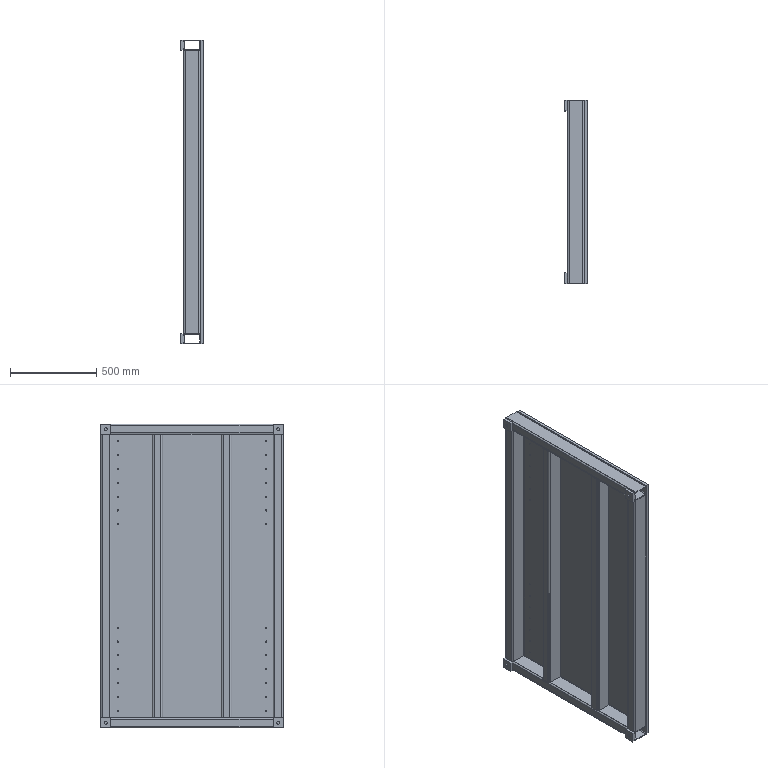Part | SolidWorks | features MirrorPattern 5, HoleWzd 3, ICE 2, LPattern 1, WeldMemberFeat 1, WeldmentFeature 1 | 9 solids | 226 faces | box 132 x 1060 x 1760 mm | volume 42498587 mm3 | cylinder 134 | plane 90 | cone 2 | commonest cylinder face diameters 6.8 x66 10 x24 20 x24 17.5 x12 8.5 x8